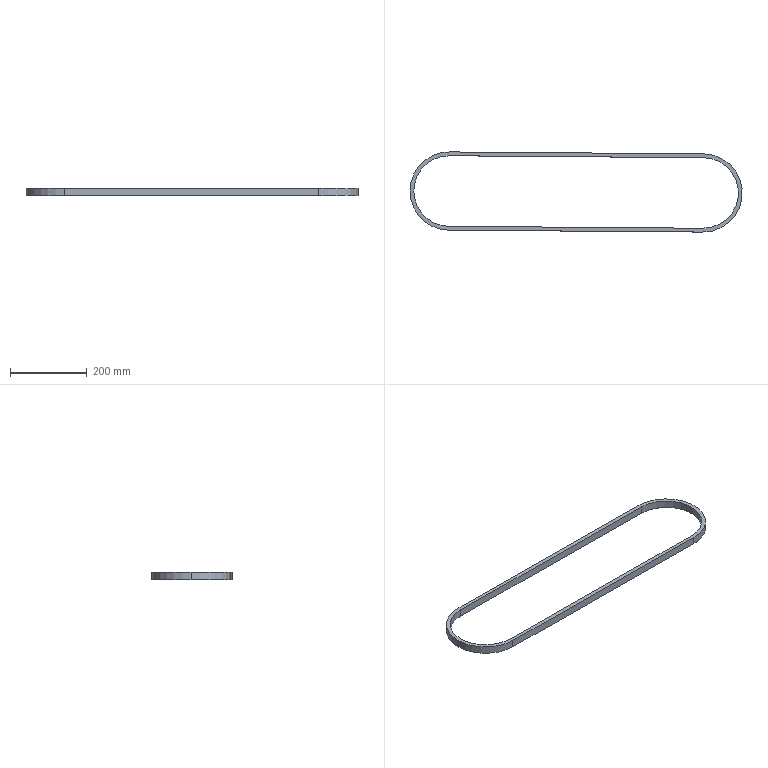Part | SolidWorks | features BeltProfileFeature 1, ExtruThin 1 | 1 solid | 12 faces | box 863.25 x 208.25 x 20 mm | volume 385430 mm3 | cylinder 6 | plane 6 | commonest cylinder face diameters 183.25 x3 203.25 x3
STEP:
#1=CARTESIAN_POINT('',(0.6941,91.622,10.));
#2=VERTEX_POINT('',#1);
#3=CARTESIAN_POINT('',(-91.625,0.,10.));
#4=VERTEX_POINT('',#3);
#5=CARTESIAN_POINT('',(0.,0.,10.));
#6=DIRECTION('',(0.,0.,1.));
#7=DIRECTION('',(-1.,0.,0.));
#8=AXIS2_PLACEMENT_3D('',#5,#6,#7);
#9=CIRCLE('',#8,91.625);
#10=EDGE_CURVE('',#2,#4,#9,.T.);
#11=ORIENTED_EDGE('',*,*,#10,.T.);
#12=CARTESIAN_POINT('',(-91.625,0.,-10.));
#13=VERTEX_POINT('',#12);
#14=CARTESIAN_POINT('',(-91.625,0.,10.));
#15=DIRECTION('',(0.,0.,-1.));
#16=VECTOR('',#15,1000.);
#17=LINE('',#14,#16);
#18=EDGE_CURVE('',#4,#13,#17,.T.);
#19=ORIENTED_EDGE('',*,*,#18,.T.);
#20=CARTESIAN_POINT('',(0.6941,91.622,-10.));
#21=VERTEX_POINT('',#20);
#22=CARTESIAN_POINT('',(0.,0.,-10.));
#23=DIRECTION('',(0.,0.,1.));
#24=DIRECTION('',(-1.,0.,0.));
#25=AXIS2_PLACEMENT_3D('',#22,#23,#24);
#26=CIRCLE('',#25,91.625);
#27=EDGE_CURVE('',#21,#13,#26,.T.);
#28=ORIENTED_EDGE('',*,*,#27,.F.);
#29=CARTESIAN_POINT('',(0.6941,91.622,10.));
#30=DIRECTION('',(0.,0.,-1.));
#31=VECTOR('',#30,1000.);
#32=LINE('',#29,#31);
#33=EDGE_CURVE('',#2,#21,#32,.T.);
#34=ORIENTED_EDGE('',*,*,#33,.F.);
#35=EDGE_LOOP('',(#11,#19,#28,#34));
#36=FACE_OUTER_BOUND('',#35,.T.);
#37=CARTESIAN_POINT('',(0.,0.,10.));
#38=DIRECTION('',(0.,0.,-1.));
#39=DIRECTION('',(-1.,0.,0.));
#40=AXIS2_PLACEMENT_3D('',#37,#38,#39);
#41=CYLINDRICAL_SURFACE('',#40,91.625);
#42=ADVANCED_FACE('',(#36),#41,.F.);
#43=CARTESIAN_POINT('',(-101.625,0.,10.));
#44=VERTEX_POINT('',#43);
#45=CARTESIAN_POINT('',(-0.7699,-101.622,10.));
#46=VERTEX_POINT('',#45);
#47=CARTESIAN_POINT('',(0.,0.,10.));
#48=DIRECTION('',(0.,0.,1.));
#49=DIRECTION('',(-1.,0.,0.));
#50=AXIS2_PLACEMENT_3D('',#47,#48,#49);
#51=CIRCLE('',#50,101.625);
#52=EDGE_CURVE('',#44,#46,#51,.T.);
#53=ORIENTED_EDGE('',*,*,#52,.F.);
#54=CARTESIAN_POINT('',(-101.625,0.,-10.));
#55=VERTEX_POINT('',#54);
#56=CARTESIAN_POINT('',(-101.625,0.,10.));
#57=DIRECTION('',(0.,0.,-1.));
#58=VECTOR('',#57,1000.);
#59=LINE('',#56,#58);
#60=EDGE_CURVE('',#44,#55,#59,.T.);
#61=ORIENTED_EDGE('',*,*,#60,.T.);
#62=CARTESIAN_POINT('',(-0.7699,-101.622,-10.));
#63=VERTEX_POINT('',#62);
#64=CARTESIAN_POINT('',(0.,0.,-10.));
#65=DIRECTION('',(0.,0.,1.));
#66=DIRECTION('',(-1.,0.,0.));
#67=AXIS2_PLACEMENT_3D('',#64,#65,#66);
#68=CIRCLE('',#67,101.625);
#69=EDGE_CURVE('',#55,#63,#68,.T.);
#70=ORIENTED_EDGE('',*,*,#69,.T.);
#71=CARTESIAN_POINT('',(-0.7699,-101.622,10.));
#72=DIRECTION('',(0.,0.,-1.));
#73=VECTOR('',#72,1000.);
#74=LINE('',#71,#73);
#75=EDGE_CURVE('',#46,#63,#74,.T.);
#76=ORIENTED_EDGE('',*,*,#75,.F.);
#77=EDGE_LOOP('',(#53,#61,#70,#76));
#78=FACE_OUTER_BOUND('',#77,.T.);
#79=CARTESIAN_POINT('',(0.,0.,10.));
#80=DIRECTION('',(0.,0.,-1.));
#81=DIRECTION('',(-1.,0.,0.));
#82=AXIS2_PLACEMENT_3D('',#79,#80,#81);
#83=CYLINDRICAL_SURFACE('',#82,101.625);
#84=ADVANCED_FACE('',(#78),#83,.T.);
#85=CARTESIAN_POINT('',(0.7699,101.622,10.));
#86=VERTEX_POINT('',#85);
#87=CARTESIAN_POINT('',(0.,0.,10.));
#88=DIRECTION('',(0.,0.,1.));
#89=DIRECTION('',(-1.,0.,0.));
#90=AXIS2_PLACEMENT_3D('',#87,#88,#89);
#91=CIRCLE('',#90,101.625);
#92=EDGE_CURVE('',#86,#44,#91,.T.);
#93=ORIENTED_EDGE('',*,*,#92,.T.);
#94=ORIENTED_EDGE('',*,*,#52,.T.);
#95=CARTESIAN_POINT('',(659.23,-106.622,10.));
#96=VERTEX_POINT('',#95);
#97=CARTESIAN_POINT('',(-0.7699,-101.622,10.));
#98=DIRECTION('',(1.,-0.007576,0.));
#99=VECTOR('',#98,1000.);
#100=LINE('',#97,#99);
#101=EDGE_CURVE('',#46,#96,#100,.T.);
#102=ORIENTED_EDGE('',*,*,#101,.T.);
#103=CARTESIAN_POINT('',(660.77,96.622,10.));
#104=VERTEX_POINT('',#103);
#105=CARTESIAN_POINT('',(660.,-5.,10.));
#106=DIRECTION('',(0.,0.,1.));
#107=DIRECTION('',(-1.,0.,0.));
#108=AXIS2_PLACEMENT_3D('',#105,#106,#107);
#109=CIRCLE('',#108,101.625);
#110=EDGE_CURVE('',#96,#104,#109,.T.);
#111=ORIENTED_EDGE('',*,*,#110,.T.);
#112=CARTESIAN_POINT('',(0.7699,101.622,10.));
#113=DIRECTION('',(-1.,0.007576,0.));
#114=VECTOR('',#113,1000.);
#115=LINE('',#112,#114);
#116=EDGE_CURVE('',#104,#86,#115,.T.);
#117=ORIENTED_EDGE('',*,*,#116,.T.);
#118=EDGE_LOOP('',(#93,#94,#102,#111,#117));
#119=FACE_OUTER_BOUND('',#118,.T.);
#120=ORIENTED_EDGE('',*,*,#10,.F.);
#121=CARTESIAN_POINT('',(660.694,86.622,10.));
#122=VERTEX_POINT('',#121);
#123=CARTESIAN_POINT('',(0.6941,91.622,10.));
#124=DIRECTION('',(-1.,0.007576,0.));
#125=VECTOR('',#124,1000.);
#126=LINE('',#123,#125);
#127=EDGE_CURVE('',#122,#2,#126,.T.);
#128=ORIENTED_EDGE('',*,*,#127,.F.);
#129=CARTESIAN_POINT('',(659.306,-96.622,10.));
#130=VERTEX_POINT('',#129);
#131=CARTESIAN_POINT('',(660.,-5.,10.));
#132=DIRECTION('',(0.,0.,1.));
#133=DIRECTION('',(-1.,0.,0.));
#134=AXIS2_PLACEMENT_3D('',#131,#132,#133);
#135=CIRCLE('',#134,91.625);
#136=EDGE_CURVE('',#130,#122,#135,.T.);
#137=ORIENTED_EDGE('',*,*,#136,.F.);
#138=CARTESIAN_POINT('',(-0.6941,-91.622,10.));
#139=VERTEX_POINT('',#138);
#140=CARTESIAN_POINT('',(659.306,-96.622,10.));
#141=DIRECTION('',(1.,-0.007576,0.));
#142=VECTOR('',#141,1000.);
#143=LINE('',#140,#142);
#144=EDGE_CURVE('',#139,#130,#143,.T.);
#145=ORIENTED_EDGE('',*,*,#144,.F.);
#146=CARTESIAN_POINT('',(0.,0.,10.));
#147=DIRECTION('',(0.,0.,1.));
#148=DIRECTION('',(-1.,0.,0.));
#149=AXIS2_PLACEMENT_3D('',#146,#147,#148);
#150=CIRCLE('',#149,91.625);
#151=EDGE_CURVE('',#4,#139,#150,.T.);
#152=ORIENTED_EDGE('',*,*,#151,.F.);
#153=EDGE_LOOP('',(#120,#128,#137,#145,#152));
#154=FACE_BOUND('',#153,.T.);
#155=CARTESIAN_POINT('',(0.,0.,10.));
#156=DIRECTION('',(0.,0.,-1.));
#157=DIRECTION('',(-1.,0.,0.));
#158=AXIS2_PLACEMENT_3D('',#155,#156,#157);
#159=PLANE('',#158);
#160=ADVANCED_FACE('',(#119,#154),#159,.F.);
#161=CARTESIAN_POINT('',(0.7699,101.622,-10.));
#162=VERTEX_POINT('',#161);
#163=CARTESIAN_POINT('',(0.,0.,-10.));
#164=DIRECTION('',(0.,0.,1.));
#165=DIRECTION('',(-1.,0.,0.));
#166=AXIS2_PLACEMENT_3D('',#163,#164,#165);
#167=CIRCLE('',#166,101.625);
#168=EDGE_CURVE('',#162,#55,#167,.T.);
#169=ORIENTED_EDGE('',*,*,#168,.F.);
#170=CARTESIAN_POINT('',(660.77,96.622,-10.));
#171=VERTEX_POINT('',#170);
#172=CARTESIAN_POINT('',(0.7699,101.622,-10.));
#173=DIRECTION('',(-1.,0.007576,0.));
#174=VECTOR('',#173,1000.);
#175=LINE('',#172,#174);
#176=EDGE_CURVE('',#171,#162,#175,.T.);
#177=ORIENTED_EDGE('',*,*,#176,.F.);
#178=CARTESIAN_POINT('',(659.23,-106.622,-10.));
#179=VERTEX_POINT('',#178);
#180=CARTESIAN_POINT('',(660.,-5.,-10.));
#181=DIRECTION('',(0.,0.,1.));
#182=DIRECTION('',(-1.,0.,0.));
#183=AXIS2_PLACEMENT_3D('',#180,#181,#182);
#184=CIRCLE('',#183,101.625);
#185=EDGE_CURVE('',#179,#171,#184,.T.);
#186=ORIENTED_EDGE('',*,*,#185,.F.);
#187=CARTESIAN_POINT('',(-0.7699,-101.622,-10.));
#188=DIRECTION('',(1.,-0.007576,0.));
#189=VECTOR('',#188,1000.);
#190=LINE('',#187,#189);
#191=EDGE_CURVE('',#63,#179,#190,.T.);
#192=ORIENTED_EDGE('',*,*,#191,.F.);
#193=ORIENTED_EDGE('',*,*,#69,.F.);
#194=EDGE_LOOP('',(#169,#177,#186,#192,#193));
#195=FACE_OUTER_BOUND('',#194,.T.);
#196=CARTESIAN_POINT('',(660.694,86.622,-10.));
#197=VERTEX_POINT('',#196);
#198=CARTESIAN_POINT('',(0.6941,91.622,-10.));
#199=DIRECTION('',(-1.,0.007576,0.));
#200=VECTOR('',#199,1000.);
#201=LINE('',#198,#200);
#202=EDGE_CURVE('',#197,#21,#201,.T.);
#203=ORIENTED_EDGE('',*,*,#202,.T.);
#204=ORIENTED_EDGE('',*,*,#27,.T.);
#205=CARTESIAN_POINT('',(-0.6941,-91.622,-10.));
#206=VERTEX_POINT('',#205);
#207=CARTESIAN_POINT('',(0.,0.,-10.));
#208=DIRECTION('',(0.,0.,1.));
#209=DIRECTION('',(-1.,0.,0.));
#210=AXIS2_PLACEMENT_3D('',#207,#208,#209);
#211=CIRCLE('',#210,91.625);
#212=EDGE_CURVE('',#13,#206,#211,.T.);
#213=ORIENTED_EDGE('',*,*,#212,.T.);
#214=CARTESIAN_POINT('',(659.306,-96.622,-10.));
#215=VERTEX_POINT('',#214);
#216=CARTESIAN_POINT('',(659.306,-96.622,-10.));
#217=DIRECTION('',(1.,-0.007576,0.));
#218=VECTOR('',#217,1000.);
#219=LINE('',#216,#218);
#220=EDGE_CURVE('',#206,#215,#219,.T.);
#221=ORIENTED_EDGE('',*,*,#220,.T.);
#222=CARTESIAN_POINT('',(660.,-5.,-10.));
#223=DIRECTION('',(0.,0.,1.));
#224=DIRECTION('',(-1.,0.,0.));
#225=AXIS2_PLACEMENT_3D('',#222,#223,#224);
#226=CIRCLE('',#225,91.625);
#227=EDGE_CURVE('',#215,#197,#226,.T.);
#228=ORIENTED_EDGE('',*,*,#227,.T.);
#229=EDGE_LOOP('',(#203,#204,#213,#221,#228));
#230=FACE_BOUND('',#229,.T.);
#231=CARTESIAN_POINT('',(0.,0.,-10.));
#232=DIRECTION('',(0.,0.,-1.));
#233=DIRECTION('',(-1.,0.,0.));
#234=AXIS2_PLACEMENT_3D('',#231,#232,#233);
#235=PLANE('',#234);
#236=ADVANCED_FACE('',(#195,#230),#235,.T.);
#237=ORIENTED_EDGE('',*,*,#60,.F.);
#238=ORIENTED_EDGE('',*,*,#92,.F.);
#239=CARTESIAN_POINT('',(0.7699,101.622,10.));
#240=DIRECTION('',(0.,0.,-1.));
#241=VECTOR('',#240,1000.);
#242=LINE('',#239,#241);
#243=EDGE_CURVE('',#86,#162,#242,.T.);
#244=ORIENTED_EDGE('',*,*,#243,.T.);
#245=ORIENTED_EDGE('',*,*,#168,.T.);
#246=EDGE_LOOP('',(#237,#238,#244,#245));
#247=FACE_OUTER_BOUND('',#246,.T.);
#248=CARTESIAN_POINT('',(0.,0.,10.));
#249=DIRECTION('',(0.,0.,-1.));
#250=DIRECTION('',(-1.,0.,0.));
#251=AXIS2_PLACEMENT_3D('',#248,#249,#250);
#252=CYLINDRICAL_SURFACE('',#251,101.625);
#253=ADVANCED_FACE('',(#247),#252,.T.);
#254=ORIENTED_EDGE('',*,*,#191,.T.);
#255=CARTESIAN_POINT('',(659.23,-106.622,10.));
#256=DIRECTION('',(0.,0.,-1.));
#257=VECTOR('',#256,1000.);
#258=LINE('',#255,#257);
#259=EDGE_CURVE('',#96,#179,#258,.T.);
#260=ORIENTED_EDGE('',*,*,#259,.F.);
#261=ORIENTED_EDGE('',*,*,#101,.F.);
#262=ORIENTED_EDGE('',*,*,#75,.T.);
#263=EDGE_LOOP('',(#254,#260,#261,#262));
#264=FACE_OUTER_BOUND('',#263,.T.);
#265=CARTESIAN_POINT('',(-0.7699,-101.622,10.));
#266=DIRECTION('',(0.007576,1.,0.));
#267=DIRECTION('',(-1.,0.007576,0.));
#268=AXIS2_PLACEMENT_3D('',#265,#266,#267);
#269=PLANE('',#268);
#270=ADVANCED_FACE('',(#264),#269,.F.);
#271=ORIENTED_EDGE('',*,*,#185,.T.);
#272=CARTESIAN_POINT('',(660.77,96.622,10.));
#273=DIRECTION('',(0.,0.,-1.));
#274=VECTOR('',#273,1000.);
#275=LINE('',#272,#274);
#276=EDGE_CURVE('',#104,#171,#275,.T.);
#277=ORIENTED_EDGE('',*,*,#276,.F.);
#278=ORIENTED_EDGE('',*,*,#110,.F.);
#279=ORIENTED_EDGE('',*,*,#259,.T.);
#280=EDGE_LOOP('',(#271,#277,#278,#279));
#281=FACE_OUTER_BOUND('',#280,.T.);
#282=CARTESIAN_POINT('',(660.,-5.,10.));
#283=DIRECTION('',(0.,0.,-1.));
#284=DIRECTION('',(-1.,0.,0.));
#285=AXIS2_PLACEMENT_3D('',#282,#283,#284);
#286=CYLINDRICAL_SURFACE('',#285,101.625);
#287=ADVANCED_FACE('',(#281),#286,.T.);
#288=ORIENTED_EDGE('',*,*,#176,.T.);
#289=ORIENTED_EDGE('',*,*,#243,.F.);
#290=ORIENTED_EDGE('',*,*,#116,.F.);
#291=ORIENTED_EDGE('',*,*,#276,.T.);
#292=EDGE_LOOP('',(#288,#289,#290,#291));
#293=FACE_OUTER_BOUND('',#292,.T.);
#294=CARTESIAN_POINT('',(0.7699,101.622,10.));
#295=DIRECTION('',(-0.007576,-1.,0.));
#296=DIRECTION('',(1.,-0.007576,0.));
#297=AXIS2_PLACEMENT_3D('',#294,#295,#296);
#298=PLANE('',#297);
#299=ADVANCED_FACE('',(#293),#298,.F.);
#300=ORIENTED_EDGE('',*,*,#18,.F.);
#301=ORIENTED_EDGE('',*,*,#151,.T.);
#302=CARTESIAN_POINT('',(-0.6941,-91.622,10.));
#303=DIRECTION('',(0.,0.,-1.));
#304=VECTOR('',#303,1000.);
#305=LINE('',#302,#304);
#306=EDGE_CURVE('',#139,#206,#305,.T.);
#307=ORIENTED_EDGE('',*,*,#306,.T.);
#308=ORIENTED_EDGE('',*,*,#212,.F.);
#309=EDGE_LOOP('',(#300,#301,#307,#308));
#310=FACE_OUTER_BOUND('',#309,.T.);
#311=CARTESIAN_POINT('',(0.,0.,10.));
#312=DIRECTION('',(0.,0.,-1.));
#313=DIRECTION('',(-1.,0.,0.));
#314=AXIS2_PLACEMENT_3D('',#311,#312,#313);
#315=CYLINDRICAL_SURFACE('',#314,91.625);
#316=ADVANCED_FACE('',(#310),#315,.F.);
#317=ORIENTED_EDGE('',*,*,#220,.F.);
#318=ORIENTED_EDGE('',*,*,#306,.F.);
#319=ORIENTED_EDGE('',*,*,#144,.T.);
#320=CARTESIAN_POINT('',(659.306,-96.622,10.));
#321=DIRECTION('',(0.,0.,-1.));
#322=VECTOR('',#321,1000.);
#323=LINE('',#320,#322);
#324=EDGE_CURVE('',#130,#215,#323,.T.);
#325=ORIENTED_EDGE('',*,*,#324,.T.);
#326=EDGE_LOOP('',(#317,#318,#319,#325));
#327=FACE_OUTER_BOUND('',#326,.T.);
#328=CARTESIAN_POINT('',(659.306,-96.622,10.));
#329=DIRECTION('',(0.007576,1.,0.));
#330=DIRECTION('',(-1.,0.007576,0.));
#331=AXIS2_PLACEMENT_3D('',#328,#329,#330);
#332=PLANE('',#331);
#333=ADVANCED_FACE('',(#327),#332,.T.);
#334=ORIENTED_EDGE('',*,*,#227,.F.);
#335=ORIENTED_EDGE('',*,*,#324,.F.);
#336=ORIENTED_EDGE('',*,*,#136,.T.);
#337=CARTESIAN_POINT('',(660.694,86.622,10.));
#338=DIRECTION('',(0.,0.,-1.));
#339=VECTOR('',#338,1000.);
#340=LINE('',#337,#339);
#341=EDGE_CURVE('',#122,#197,#340,.T.);
#342=ORIENTED_EDGE('',*,*,#341,.T.);
#343=EDGE_LOOP('',(#334,#335,#336,#342));
#344=FACE_OUTER_BOUND('',#343,.T.);
#345=CARTESIAN_POINT('',(660.,-5.,10.));
#346=DIRECTION('',(0.,0.,-1.));
#347=DIRECTION('',(-1.,0.,0.));
#348=AXIS2_PLACEMENT_3D('',#345,#346,#347);
#349=CYLINDRICAL_SURFACE('',#348,91.625);
#350=ADVANCED_FACE('',(#344),#349,.F.);
#351=ORIENTED_EDGE('',*,*,#202,.F.);
#352=ORIENTED_EDGE('',*,*,#341,.F.);
#353=ORIENTED_EDGE('',*,*,#127,.T.);
#354=ORIENTED_EDGE('',*,*,#33,.T.);
#355=EDGE_LOOP('',(#351,#352,#353,#354));
#356=FACE_OUTER_BOUND('',#355,.T.);
#357=CARTESIAN_POINT('',(0.6941,91.622,10.));
#358=DIRECTION('',(-0.007576,-1.,0.));
#359=DIRECTION('',(1.,-0.007576,0.));
#360=AXIS2_PLACEMENT_3D('',#357,#358,#359);
#361=PLANE('',#360);
#362=ADVANCED_FACE('',(#356),#361,.T.);
#363=CLOSED_SHELL('',(#42,#84,#160,#236,#253,#270,#287,#299,#316,#333,#350,#362));
#364=MANIFOLD_SOLID_BREP('',#363);
#365=CARTESIAN_POINT('',(0.,0.,0.));
#366=DIRECTION('',(0.,0.,1.));
#367=DIRECTION('',(1.,0.,0.));
#368=AXIS2_PLACEMENT_3D('',#365,#366,#367);
#369=(LENGTH_UNIT()NAMED_UNIT(*)SI_UNIT(.MILLI.,.METRE.));
#370=UNCERTAINTY_MEASURE_WITH_UNIT(LENGTH_MEASURE(0.00001),#369,'','');
#371=(NAMED_UNIT(*)PLANE_ANGLE_UNIT()SI_UNIT($,.RADIAN.));
#372=(NAMED_UNIT(*)SI_UNIT($,.STERADIAN.)SOLID_ANGLE_UNIT());
#373=(GEOMETRIC_REPRESENTATION_CONTEXT(3)GLOBAL_UNCERTAINTY_ASSIGNED_CONTEXT((#370))GLOBAL_UNIT_ASSIGNED_CONTEXT((#369,#371,#372))REPRESENTATION_CONTEXT('',''));
#374=ADVANCED_BREP_SHAPE_REPRESENTATION('',(#364,#368),#373);